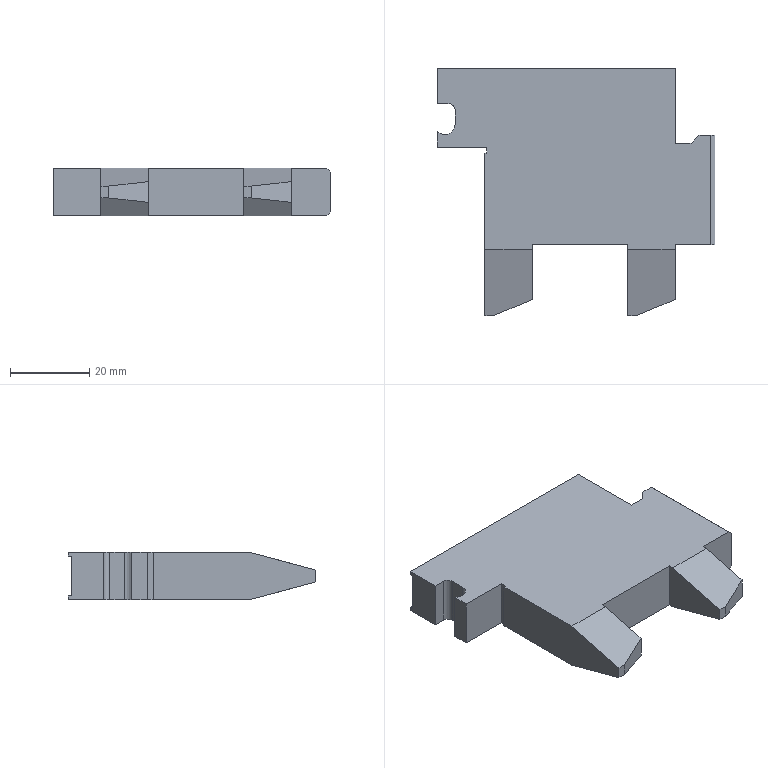Part | SolidWorks | features ICE 2, Chamfer 1, Extrusion 1 | 1 solid | 38 faces | box 70 x 62.5 x 12 mm | volume 33880 mm3 | plane 36 | cylinder 2 | commonest cylinder face diameters 3 x1 5 x1
STEP:
#1=CARTESIAN_POINT('',(0.,20.,-5.));
#2=VERTEX_POINT('',#1);
#3=CARTESIAN_POINT('',(0.,20.,-6.));
#4=VERTEX_POINT('',#3);
#5=CARTESIAN_POINT('',(0.,20.,6.));
#6=DIRECTION('',(0.,0.,-1.));
#7=VECTOR('',#6,1000.);
#8=LINE('',#5,#7);
#9=EDGE_CURVE('',#2,#4,#8,.T.);
#10=ORIENTED_EDGE('',*,*,#9,.F.);
#11=CARTESIAN_POINT('',(60.,20.,-5.));
#12=VERTEX_POINT('',#11);
#13=CARTESIAN_POINT('',(0.,20.,-5.));
#14=DIRECTION('',(-1.,0.,0.));
#15=VECTOR('',#14,1000.);
#16=LINE('',#13,#15);
#17=EDGE_CURVE('',#12,#2,#16,.T.);
#18=ORIENTED_EDGE('',*,*,#17,.F.);
#19=CARTESIAN_POINT('',(60.,20.,-6.));
#20=VERTEX_POINT('',#19);
#21=CARTESIAN_POINT('',(60.,20.,6.));
#22=DIRECTION('',(0.,0.,-1.));
#23=VECTOR('',#22,1000.);
#24=LINE('',#21,#23);
#25=EDGE_CURVE('',#12,#20,#24,.T.);
#26=ORIENTED_EDGE('',*,*,#25,.T.);
#27=CARTESIAN_POINT('',(0.,20.,-6.));
#28=DIRECTION('',(-1.,0.,0.));
#29=VECTOR('',#28,1000.);
#30=LINE('',#27,#29);
#31=EDGE_CURVE('',#20,#4,#30,.T.);
#32=ORIENTED_EDGE('',*,*,#31,.T.);
#33=EDGE_LOOP('',(#10,#18,#26,#32));
#34=FACE_OUTER_BOUND('',#33,.T.);
#35=CARTESIAN_POINT('',(0.,20.,6.));
#36=DIRECTION('',(0.,-1.,0.));
#37=DIRECTION('',(1.,0.,0.));
#38=AXIS2_PLACEMENT_3D('',#35,#36,#37);
#39=PLANE('',#38);
#40=ADVANCED_FACE('',(#34),#39,.F.);
#41=CARTESIAN_POINT('',(0.,0.,-6.));
#42=VERTEX_POINT('',#41);
#43=CARTESIAN_POINT('',(12.5,0.,-6.));
#44=VERTEX_POINT('',#43);
#45=CARTESIAN_POINT('',(12.5,0.,-6.));
#46=DIRECTION('',(1.,0.,0.));
#47=VECTOR('',#46,1000.);
#48=LINE('',#45,#47);
#49=EDGE_CURVE('',#42,#44,#48,.T.);
#50=ORIENTED_EDGE('',*,*,#49,.T.);
#51=CARTESIAN_POINT('',(12.5,0.,6.));
#52=VERTEX_POINT('',#51);
#53=CARTESIAN_POINT('',(12.5,0.,6.));
#54=DIRECTION('',(0.,0.,-1.));
#55=VECTOR('',#54,1000.);
#56=LINE('',#53,#55);
#57=EDGE_CURVE('',#52,#44,#56,.T.);
#58=ORIENTED_EDGE('',*,*,#57,.F.);
#59=CARTESIAN_POINT('',(0.,0.,6.));
#60=VERTEX_POINT('',#59);
#61=CARTESIAN_POINT('',(12.5,0.,6.));
#62=DIRECTION('',(1.,0.,0.));
#63=VECTOR('',#62,1000.);
#64=LINE('',#61,#63);
#65=EDGE_CURVE('',#60,#52,#64,.T.);
#66=ORIENTED_EDGE('',*,*,#65,.F.);
#67=CARTESIAN_POINT('',(0.,0.,6.));
#68=DIRECTION('',(0.,0.,-1.));
#69=VECTOR('',#68,1000.);
#70=LINE('',#67,#69);
#71=EDGE_CURVE('',#60,#42,#70,.T.);
#72=ORIENTED_EDGE('',*,*,#71,.T.);
#73=EDGE_LOOP('',(#50,#58,#66,#72));
#74=FACE_OUTER_BOUND('',#73,.T.);
#75=CARTESIAN_POINT('',(12.5,0.,6.));
#76=DIRECTION('',(0.,1.,0.));
#77=DIRECTION('',(-1.,0.,0.));
#78=AXIS2_PLACEMENT_3D('',#75,#76,#77);
#79=PLANE('',#78);
#80=ADVANCED_FACE('',(#74),#79,.F.);
#81=CARTESIAN_POINT('',(12.5,-1.5,-6.));
#82=VERTEX_POINT('',#81);
#83=CARTESIAN_POINT('',(12.5,0.,-6.));
#84=DIRECTION('',(0.,-1.,0.));
#85=VECTOR('',#84,1000.);
#86=LINE('',#83,#85);
#87=EDGE_CURVE('',#44,#82,#86,.T.);
#88=ORIENTED_EDGE('',*,*,#87,.T.);
#89=CARTESIAN_POINT('',(12.5,-1.5,6.));
#90=VERTEX_POINT('',#89);
#91=CARTESIAN_POINT('',(12.5,-1.5,6.));
#92=DIRECTION('',(0.,0.,-1.));
#93=VECTOR('',#92,1000.);
#94=LINE('',#91,#93);
#95=EDGE_CURVE('',#90,#82,#94,.T.);
#96=ORIENTED_EDGE('',*,*,#95,.F.);
#97=CARTESIAN_POINT('',(12.5,0.,6.));
#98=DIRECTION('',(0.,-1.,0.));
#99=VECTOR('',#98,1000.);
#100=LINE('',#97,#99);
#101=EDGE_CURVE('',#52,#90,#100,.T.);
#102=ORIENTED_EDGE('',*,*,#101,.F.);
#103=ORIENTED_EDGE('',*,*,#57,.T.);
#104=EDGE_LOOP('',(#88,#96,#102,#103));
#105=FACE_OUTER_BOUND('',#104,.T.);
#106=CARTESIAN_POINT('',(12.5,0.,6.));
#107=DIRECTION('',(1.,0.,0.));
#108=DIRECTION('',(0.,0.,-1.));
#109=AXIS2_PLACEMENT_3D('',#106,#107,#108);
#110=PLANE('',#109);
#111=ADVANCED_FACE('',(#105),#110,.F.);
#112=CARTESIAN_POINT('',(12.,-1.5,-6.));
#113=VERTEX_POINT('',#112);
#114=CARTESIAN_POINT('',(12.5,-1.5,-6.));
#115=DIRECTION('',(-1.,0.,0.));
#116=VECTOR('',#115,1000.);
#117=LINE('',#114,#116);
#118=EDGE_CURVE('',#82,#113,#117,.T.);
#119=ORIENTED_EDGE('',*,*,#118,.T.);
#120=CARTESIAN_POINT('',(12.,-1.5,6.));
#121=VERTEX_POINT('',#120);
#122=CARTESIAN_POINT('',(12.,-1.5,6.));
#123=DIRECTION('',(0.,0.,-1.));
#124=VECTOR('',#123,1000.);
#125=LINE('',#122,#124);
#126=EDGE_CURVE('',#121,#113,#125,.T.);
#127=ORIENTED_EDGE('',*,*,#126,.F.);
#128=CARTESIAN_POINT('',(12.5,-1.5,6.));
#129=DIRECTION('',(-1.,0.,0.));
#130=VECTOR('',#129,1000.);
#131=LINE('',#128,#130);
#132=EDGE_CURVE('',#90,#121,#131,.T.);
#133=ORIENTED_EDGE('',*,*,#132,.F.);
#134=ORIENTED_EDGE('',*,*,#95,.T.);
#135=EDGE_LOOP('',(#119,#127,#133,#134));
#136=FACE_OUTER_BOUND('',#135,.T.);
#137=CARTESIAN_POINT('',(12.5,-1.5,6.));
#138=DIRECTION('',(0.,-1.,0.));
#139=DIRECTION('',(0.,0.,-1.));
#140=AXIS2_PLACEMENT_3D('',#137,#138,#139);
#141=PLANE('',#140);
#142=ADVANCED_FACE('',(#136),#141,.F.);
#143=CARTESIAN_POINT('',(12.,-25.706,-6.));
#144=VERTEX_POINT('',#143);
#145=CARTESIAN_POINT('',(12.,-1.5,-6.));
#146=DIRECTION('',(0.,-1.,0.));
#147=VECTOR('',#146,1000.);
#148=LINE('',#145,#147);
#149=EDGE_CURVE('',#113,#144,#148,.T.);
#150=ORIENTED_EDGE('',*,*,#149,.T.);
#151=CARTESIAN_POINT('',(12.,-42.5,-1.5));
#152=VERTEX_POINT('',#151);
#153=CARTESIAN_POINT('',(12.,-42.5,-1.5));
#154=DIRECTION('',(0.,0.9659,-0.2588));
#155=VECTOR('',#154,1000.);
#156=LINE('',#153,#155);
#157=EDGE_CURVE('',#152,#144,#156,.T.);
#158=ORIENTED_EDGE('',*,*,#157,.F.);
#159=CARTESIAN_POINT('',(12.,-42.5,1.5));
#160=VERTEX_POINT('',#159);
#161=CARTESIAN_POINT('',(12.,-42.5,6.));
#162=DIRECTION('',(0.,0.,-1.));
#163=VECTOR('',#162,1000.);
#164=LINE('',#161,#163);
#165=EDGE_CURVE('',#160,#152,#164,.T.);
#166=ORIENTED_EDGE('',*,*,#165,.F.);
#167=CARTESIAN_POINT('',(12.,-25.706,6.));
#168=VERTEX_POINT('',#167);
#169=CARTESIAN_POINT('',(12.,-42.5,1.5));
#170=DIRECTION('',(0.,-0.9659,-0.2588));
#171=VECTOR('',#170,1000.);
#172=LINE('',#169,#171);
#173=EDGE_CURVE('',#168,#160,#172,.T.);
#174=ORIENTED_EDGE('',*,*,#173,.F.);
#175=CARTESIAN_POINT('',(12.,-1.5,6.));
#176=DIRECTION('',(0.,-1.,0.));
#177=VECTOR('',#176,1000.);
#178=LINE('',#175,#177);
#179=EDGE_CURVE('',#121,#168,#178,.T.);
#180=ORIENTED_EDGE('',*,*,#179,.F.);
#181=ORIENTED_EDGE('',*,*,#126,.T.);
#182=EDGE_LOOP('',(#150,#158,#166,#174,#180,#181));
#183=FACE_OUTER_BOUND('',#182,.T.);
#184=CARTESIAN_POINT('',(12.,-1.5,6.));
#185=DIRECTION('',(1.,0.,0.));
#186=DIRECTION('',(0.,1.,0.));
#187=AXIS2_PLACEMENT_3D('',#184,#185,#186);
#188=PLANE('',#187);
#189=ADVANCED_FACE('',(#183),#188,.F.);
#190=ORIENTED_EDGE('',*,*,#165,.T.);
#191=CARTESIAN_POINT('',(14.,-42.5,-1.5));
#192=VERTEX_POINT('',#191);
#193=CARTESIAN_POINT('',(70.,-42.5,-1.5));
#194=DIRECTION('',(-1.,0.,0.));
#195=VECTOR('',#194,1000.);
#196=LINE('',#193,#195);
#197=EDGE_CURVE('',#192,#152,#196,.T.);
#198=ORIENTED_EDGE('',*,*,#197,.F.);
#199=CARTESIAN_POINT('',(14.,-42.5,1.5));
#200=VERTEX_POINT('',#199);
#201=CARTESIAN_POINT('',(14.,-42.5,6.));
#202=DIRECTION('',(0.,0.,-1.));
#203=VECTOR('',#202,1000.);
#204=LINE('',#201,#203);
#205=EDGE_CURVE('',#200,#192,#204,.T.);
#206=ORIENTED_EDGE('',*,*,#205,.F.);
#207=CARTESIAN_POINT('',(70.,-42.5,1.5));
#208=DIRECTION('',(-1.,0.,0.));
#209=VECTOR('',#208,1000.);
#210=LINE('',#207,#209);
#211=EDGE_CURVE('',#200,#160,#210,.T.);
#212=ORIENTED_EDGE('',*,*,#211,.T.);
#213=EDGE_LOOP('',(#190,#198,#206,#212));
#214=FACE_OUTER_BOUND('',#213,.T.);
#215=CARTESIAN_POINT('',(14.,-42.5,6.));
#216=DIRECTION('',(0.,1.,0.));
#217=DIRECTION('',(0.,0.,1.));
#218=AXIS2_PLACEMENT_3D('',#215,#216,#217);
#219=PLANE('',#218);
#220=ADVANCED_FACE('',(#214),#219,.F.);
#221=ORIENTED_EDGE('',*,*,#205,.T.);
#222=CARTESIAN_POINT('',(24.,-38.358,-2.61));
#223=VERTEX_POINT('',#222);
#224=CARTESIAN_POINT('',(23.193,-38.692,-2.52));
#225=DIRECTION('',(0.9191,0.3807,-0.102));
#226=VECTOR('',#225,1000.);
#227=LINE('',#224,#226);
#228=EDGE_CURVE('',#192,#223,#227,.T.);
#229=ORIENTED_EDGE('',*,*,#228,.T.);
#230=CARTESIAN_POINT('',(24.,-38.358,2.61));
#231=VERTEX_POINT('',#230);
#232=CARTESIAN_POINT('',(24.,-38.358,6.));
#233=DIRECTION('',(0.,0.,-1.));
#234=VECTOR('',#233,1000.);
#235=LINE('',#232,#234);
#236=EDGE_CURVE('',#231,#223,#235,.T.);
#237=ORIENTED_EDGE('',*,*,#236,.F.);
#238=CARTESIAN_POINT('',(24.318,-38.226,2.645));
#239=DIRECTION('',(-0.9191,-0.3807,-0.102));
#240=VECTOR('',#239,1000.);
#241=LINE('',#238,#240);
#242=EDGE_CURVE('',#231,#200,#241,.T.);
#243=ORIENTED_EDGE('',*,*,#242,.T.);
#244=EDGE_LOOP('',(#221,#229,#237,#243));
#245=FACE_OUTER_BOUND('',#244,.T.);
#246=CARTESIAN_POINT('',(24.,-38.358,6.));
#247=DIRECTION('',(-0.3827,0.9239,0.));
#248=DIRECTION('',(-0.9239,-0.3827,0.));
#249=AXIS2_PLACEMENT_3D('',#246,#247,#248);
#250=PLANE('',#249);
#251=ADVANCED_FACE('',(#245),#250,.F.);
#252=ORIENTED_EDGE('',*,*,#236,.T.);
#253=CARTESIAN_POINT('',(24.,-25.706,-6.));
#254=VERTEX_POINT('',#253);
#255=CARTESIAN_POINT('',(24.,-27.581,-5.498));
#256=DIRECTION('',(0.,0.9659,-0.2588));
#257=VECTOR('',#256,1000.);
#258=LINE('',#255,#257);
#259=EDGE_CURVE('',#223,#254,#258,.T.);
#260=ORIENTED_EDGE('',*,*,#259,.T.);
#261=CARTESIAN_POINT('',(24.,-24.5,-6.));
#262=VERTEX_POINT('',#261);
#263=CARTESIAN_POINT('',(24.,-24.5,-6.));
#264=DIRECTION('',(0.,1.,0.));
#265=VECTOR('',#264,1000.);
#266=LINE('',#263,#265);
#267=EDGE_CURVE('',#254,#262,#266,.T.);
#268=ORIENTED_EDGE('',*,*,#267,.T.);
#269=CARTESIAN_POINT('',(24.,-24.5,6.));
#270=VERTEX_POINT('',#269);
#271=CARTESIAN_POINT('',(24.,-24.5,6.));
#272=DIRECTION('',(0.,0.,-1.));
#273=VECTOR('',#272,1000.);
#274=LINE('',#271,#273);
#275=EDGE_CURVE('',#270,#262,#274,.T.);
#276=ORIENTED_EDGE('',*,*,#275,.F.);
#277=CARTESIAN_POINT('',(24.,-25.706,6.));
#278=VERTEX_POINT('',#277);
#279=CARTESIAN_POINT('',(24.,-24.5,6.));
#280=DIRECTION('',(0.,1.,0.));
#281=VECTOR('',#280,1000.);
#282=LINE('',#279,#281);
#283=EDGE_CURVE('',#278,#270,#282,.T.);
#284=ORIENTED_EDGE('',*,*,#283,.F.);
#285=CARTESIAN_POINT('',(24.,-24.581,6.301));
#286=DIRECTION('',(0.,-0.9659,-0.2588));
#287=VECTOR('',#286,1000.);
#288=LINE('',#285,#287);
#289=EDGE_CURVE('',#278,#231,#288,.T.);
#290=ORIENTED_EDGE('',*,*,#289,.T.);
#291=EDGE_LOOP('',(#252,#260,#268,#276,#284,#290));
#292=FACE_OUTER_BOUND('',#291,.T.);
#293=CARTESIAN_POINT('',(24.,-24.5,6.));
#294=DIRECTION('',(-1.,0.,0.));
#295=DIRECTION('',(0.,0.,1.));
#296=AXIS2_PLACEMENT_3D('',#293,#294,#295);
#297=PLANE('',#296);
#298=ADVANCED_FACE('',(#292),#297,.F.);
#299=CARTESIAN_POINT('',(48.,-24.5,-6.));
#300=VERTEX_POINT('',#299);
#301=CARTESIAN_POINT('',(48.,-24.5,-6.));
#302=DIRECTION('',(1.,0.,0.));
#303=VECTOR('',#302,1000.);
#304=LINE('',#301,#303);
#305=EDGE_CURVE('',#262,#300,#304,.T.);
#306=ORIENTED_EDGE('',*,*,#305,.T.);
#307=CARTESIAN_POINT('',(48.,-24.5,6.));
#308=VERTEX_POINT('',#307);
#309=CARTESIAN_POINT('',(48.,-24.5,6.));
#310=DIRECTION('',(0.,0.,-1.));
#311=VECTOR('',#310,1000.);
#312=LINE('',#309,#311);
#313=EDGE_CURVE('',#308,#300,#312,.T.);
#314=ORIENTED_EDGE('',*,*,#313,.F.);
#315=CARTESIAN_POINT('',(48.,-24.5,6.));
#316=DIRECTION('',(1.,0.,0.));
#317=VECTOR('',#316,1000.);
#318=LINE('',#315,#317);
#319=EDGE_CURVE('',#270,#308,#318,.T.);
#320=ORIENTED_EDGE('',*,*,#319,.F.);
#321=ORIENTED_EDGE('',*,*,#275,.T.);
#322=EDGE_LOOP('',(#306,#314,#320,#321));
#323=FACE_OUTER_BOUND('',#322,.T.);
#324=CARTESIAN_POINT('',(48.,-24.5,6.));
#325=DIRECTION('',(0.,1.,0.));
#326=DIRECTION('',(-1.,0.,0.));
#327=AXIS2_PLACEMENT_3D('',#324,#325,#326);
#328=PLANE('',#327);
#329=ADVANCED_FACE('',(#323),#328,.F.);
#330=CARTESIAN_POINT('',(48.,-25.706,-6.));
#331=VERTEX_POINT('',#330);
#332=CARTESIAN_POINT('',(48.,-42.5,-6.));
#333=DIRECTION('',(0.,-1.,0.));
#334=VECTOR('',#333,1000.);
#335=LINE('',#332,#334);
#336=EDGE_CURVE('',#300,#331,#335,.T.);
#337=ORIENTED_EDGE('',*,*,#336,.T.);
#338=CARTESIAN_POINT('',(48.,-42.5,-1.5));
#339=VERTEX_POINT('',#338);
#340=CARTESIAN_POINT('',(48.,-44.375,-0.9976));
#341=DIRECTION('',(0.,-0.9659,0.2588));
#342=VECTOR('',#341,1000.);
#343=LINE('',#340,#342);
#344=EDGE_CURVE('',#331,#339,#343,.T.);
#345=ORIENTED_EDGE('',*,*,#344,.T.);
#346=CARTESIAN_POINT('',(48.,-42.5,1.5));
#347=VERTEX_POINT('',#346);
#348=CARTESIAN_POINT('',(48.,-42.5,6.));
#349=DIRECTION('',(0.,0.,-1.));
#350=VECTOR('',#349,1000.);
#351=LINE('',#348,#350);
#352=EDGE_CURVE('',#347,#339,#351,.T.);
#353=ORIENTED_EDGE('',*,*,#352,.F.);
#354=CARTESIAN_POINT('',(48.,-25.706,6.));
#355=VERTEX_POINT('',#354);
#356=CARTESIAN_POINT('',(48.,-41.375,1.801));
#357=DIRECTION('',(0.,0.9659,0.2588));
#358=VECTOR('',#357,1000.);
#359=LINE('',#356,#358);
#360=EDGE_CURVE('',#347,#355,#359,.T.);
#361=ORIENTED_EDGE('',*,*,#360,.T.);
#362=CARTESIAN_POINT('',(48.,-42.5,6.));
#363=DIRECTION('',(0.,-1.,0.));
#364=VECTOR('',#363,1000.);
#365=LINE('',#362,#364);
#366=EDGE_CURVE('',#308,#355,#365,.T.);
#367=ORIENTED_EDGE('',*,*,#366,.F.);
#368=ORIENTED_EDGE('',*,*,#313,.T.);
#369=EDGE_LOOP('',(#337,#345,#353,#361,#367,#368));
#370=FACE_OUTER_BOUND('',#369,.T.);
#371=CARTESIAN_POINT('',(48.,-42.5,6.));
#372=DIRECTION('',(1.,0.,0.));
#373=DIRECTION('',(0.,0.,-1.));
#374=AXIS2_PLACEMENT_3D('',#371,#372,#373);
#375=PLANE('',#374);
#376=ADVANCED_FACE('',(#370),#375,.F.);
#377=ORIENTED_EDGE('',*,*,#352,.T.);
#378=CARTESIAN_POINT('',(50.,-42.5,-1.5));
#379=VERTEX_POINT('',#378);
#380=CARTESIAN_POINT('',(70.,-42.5,-1.5));
#381=DIRECTION('',(-1.,0.,0.));
#382=VECTOR('',#381,1000.);
#383=LINE('',#380,#382);
#384=EDGE_CURVE('',#379,#339,#383,.T.);
#385=ORIENTED_EDGE('',*,*,#384,.F.);
#386=CARTESIAN_POINT('',(50.,-42.5,1.5));
#387=VERTEX_POINT('',#386);
#388=CARTESIAN_POINT('',(50.,-42.5,6.));
#389=DIRECTION('',(0.,0.,-1.));
#390=VECTOR('',#389,1000.);
#391=LINE('',#388,#390);
#392=EDGE_CURVE('',#387,#379,#391,.T.);
#393=ORIENTED_EDGE('',*,*,#392,.F.);
#394=CARTESIAN_POINT('',(70.,-42.5,1.5));
#395=DIRECTION('',(-1.,0.,0.));
#396=VECTOR('',#395,1000.);
#397=LINE('',#394,#396);
#398=EDGE_CURVE('',#387,#347,#397,.T.);
#399=ORIENTED_EDGE('',*,*,#398,.T.);
#400=EDGE_LOOP('',(#377,#385,#393,#399));
#401=FACE_OUTER_BOUND('',#400,.T.);
#402=CARTESIAN_POINT('',(50.,-42.5,6.));
#403=DIRECTION('',(0.,1.,0.));
#404=DIRECTION('',(-1.,0.,0.));
#405=AXIS2_PLACEMENT_3D('',#402,#403,#404);
#406=PLANE('',#405);
#407=ADVANCED_FACE('',(#401),#406,.F.);
#408=ORIENTED_EDGE('',*,*,#392,.T.);
#409=CARTESIAN_POINT('',(60.,-38.358,-2.61));
#410=VERTEX_POINT('',#409);
#411=CARTESIAN_POINT('',(59.193,-38.692,-2.52));
#412=DIRECTION('',(0.9191,0.3807,-0.102));
#413=VECTOR('',#412,1000.);
#414=LINE('',#411,#413);
#415=EDGE_CURVE('',#379,#410,#414,.T.);
#416=ORIENTED_EDGE('',*,*,#415,.T.);
#417=CARTESIAN_POINT('',(60.,-38.358,2.61));
#418=VERTEX_POINT('',#417);
#419=CARTESIAN_POINT('',(60.,-38.358,6.));
#420=DIRECTION('',(0.,0.,-1.));
#421=VECTOR('',#420,1000.);
#422=LINE('',#419,#421);
#423=EDGE_CURVE('',#418,#410,#422,.T.);
#424=ORIENTED_EDGE('',*,*,#423,.F.);
#425=CARTESIAN_POINT('',(60.318,-38.226,2.645));
#426=DIRECTION('',(-0.9191,-0.3807,-0.102));
#427=VECTOR('',#426,1000.);
#428=LINE('',#425,#427);
#429=EDGE_CURVE('',#418,#387,#428,.T.);
#430=ORIENTED_EDGE('',*,*,#429,.T.);
#431=EDGE_LOOP('',(#408,#416,#424,#430));
#432=FACE_OUTER_BOUND('',#431,.T.);
#433=CARTESIAN_POINT('',(60.,-38.358,6.));
#434=DIRECTION('',(-0.3827,0.9239,0.));
#435=DIRECTION('',(-0.9239,-0.3827,0.));
#436=AXIS2_PLACEMENT_3D('',#433,#434,#435);
#437=PLANE('',#436);
#438=ADVANCED_FACE('',(#432),#437,.F.);
#439=ORIENTED_EDGE('',*,*,#423,.T.);
#440=CARTESIAN_POINT('',(60.,-25.706,-6.));
#441=VERTEX_POINT('',#440);
#442=CARTESIAN_POINT('',(60.,-40.51,-2.033));
#443=DIRECTION('',(0.,0.9659,-0.2588));
#444=VECTOR('',#443,1000.);
#445=LINE('',#442,#444);
#446=EDGE_CURVE('',#410,#441,#445,.T.);
#447=ORIENTED_EDGE('',*,*,#446,.T.);
#448=CARTESIAN_POINT('',(60.,-24.5,-6.));
#449=VERTEX_POINT('',#448);
#450=CARTESIAN_POINT('',(60.,-38.358,-6.));
#451=DIRECTION('',(0.,1.,0.));
#452=VECTOR('',#451,1000.);
#453=LINE('',#450,#452);
#454=EDGE_CURVE('',#441,#449,#453,.T.);
#455=ORIENTED_EDGE('',*,*,#454,.T.);
#456=CARTESIAN_POINT('',(60.,-24.5,6.));
#457=VERTEX_POINT('',#456);
#458=CARTESIAN_POINT('',(60.,-24.5,6.));
#459=DIRECTION('',(0.,0.,-1.));
#460=VECTOR('',#459,1000.);
#461=LINE('',#458,#460);
#462=EDGE_CURVE('',#457,#449,#461,.T.);
#463=ORIENTED_EDGE('',*,*,#462,.F.);
#464=CARTESIAN_POINT('',(60.,-25.706,6.));
#465=VERTEX_POINT('',#464);
#466=CARTESIAN_POINT('',(60.,-38.358,6.));
#467=DIRECTION('',(0.,1.,0.));
#468=VECTOR('',#467,1000.);
#469=LINE('',#466,#468);
#470=EDGE_CURVE('',#465,#457,#469,.T.);
#471=ORIENTED_EDGE('',*,*,#470,.F.);
#472=CARTESIAN_POINT('',(60.,-37.51,2.837));
#473=DIRECTION('',(0.,-0.9659,-0.2588));
#474=VECTOR('',#473,1000.);
#475=LINE('',#472,#474);
#476=EDGE_CURVE('',#465,#418,#475,.T.);
#477=ORIENTED_EDGE('',*,*,#476,.T.);
#478=EDGE_LOOP('',(#439,#447,#455,#463,#471,#477));
#479=FACE_OUTER_BOUND('',#478,.T.);
#480=CARTESIAN_POINT('',(60.,-38.358,6.));
#481=DIRECTION('',(-1.,0.,0.));
#482=DIRECTION('',(0.,0.,1.));
#483=AXIS2_PLACEMENT_3D('',#480,#481,#482);
#484=PLANE('',#483);
#485=ADVANCED_FACE('',(#479),#484,.F.);
#486=CARTESIAN_POINT('',(69.,-24.5,-6.));
#487=VERTEX_POINT('',#486);
#488=CARTESIAN_POINT('',(70.,-24.5,-6.));
#489=DIRECTION('',(1.,0.,0.));
#490=VECTOR('',#489,1000.);
#491=LINE('',#488,#490);
#492=EDGE_CURVE('',#449,#487,#491,.T.);
#493=ORIENTED_EDGE('',*,*,#492,.T.);
#494=CARTESIAN_POINT('',(70.,-24.5,-5.));
#495=VERTEX_POINT('',#494);
#496=CARTESIAN_POINT('',(70.,-24.5,-5.));
#497=DIRECTION('',(0.7071,0.,0.7071));
#498=VECTOR('',#497,1000.);
#499=LINE('',#496,#498);
#500=EDGE_CURVE('',#487,#495,#499,.T.);
#501=ORIENTED_EDGE('',*,*,#500,.T.);
#502=CARTESIAN_POINT('',(70.,-24.5,5.));
#503=VERTEX_POINT('',#502);
#504=CARTESIAN_POINT('',(70.,-24.5,6.));
#505=DIRECTION('',(0.,0.,-1.));
#506=VECTOR('',#505,1000.);
#507=LINE('',#504,#506);
#508=EDGE_CURVE('',#503,#495,#507,.T.);
#509=ORIENTED_EDGE('',*,*,#508,.F.);
#510=CARTESIAN_POINT('',(69.,-24.5,6.));
#511=VERTEX_POINT('',#510);
#512=CARTESIAN_POINT('',(69.,-24.5,6.));
#513=DIRECTION('',(-0.7071,0.,0.7071));
#514=VECTOR('',#513,1000.);
#515=LINE('',#512,#514);
#516=EDGE_CURVE('',#503,#511,#515,.T.);
#517=ORIENTED_EDGE('',*,*,#516,.T.);
#518=CARTESIAN_POINT('',(70.,-24.5,6.));
#519=DIRECTION('',(1.,0.,0.));
#520=VECTOR('',#519,1000.);
#521=LINE('',#518,#520);
#522=EDGE_CURVE('',#457,#511,#521,.T.);
#523=ORIENTED_EDGE('',*,*,#522,.F.);
#524=ORIENTED_EDGE('',*,*,#462,.T.);
#525=EDGE_LOOP('',(#493,#501,#509,#517,#523,#524));
#526=FACE_OUTER_BOUND('',#525,.T.);
#527=CARTESIAN_POINT('',(70.,-24.5,6.));
#528=DIRECTION('',(0.,1.,0.));
#529=DIRECTION('',(-1.,0.,0.));
#530=AXIS2_PLACEMENT_3D('',#527,#528,#529);
#531=PLANE('',#530);
#532=ADVANCED_FACE('',(#526),#531,.F.);
#533=ORIENTED_EDGE('',*,*,#508,.T.);
#534=CARTESIAN_POINT('',(70.,3.,-5.));
#535=VERTEX_POINT('',#534);
#536=CARTESIAN_POINT('',(70.,3.,-5.));
#537=DIRECTION('',(0.,1.,0.));
#538=VECTOR('',#537,1000.);
#539=LINE('',#536,#538);
#540=EDGE_CURVE('',#495,#535,#539,.T.);
#541=ORIENTED_EDGE('',*,*,#540,.T.);
#542=CARTESIAN_POINT('',(70.,3.,5.));
#543=VERTEX_POINT('',#542);
#544=CARTESIAN_POINT('',(70.,3.,6.));
#545=DIRECTION('',(0.,0.,-1.));
#546=VECTOR('',#545,1000.);
#547=LINE('',#544,#546);
#548=EDGE_CURVE('',#543,#535,#547,.T.);
#549=ORIENTED_EDGE('',*,*,#548,.F.);
#550=CARTESIAN_POINT('',(70.,-24.5,5.));
#551=DIRECTION('',(0.,-1.,0.));
#552=VECTOR('',#551,1000.);
#553=LINE('',#550,#552);
#554=EDGE_CURVE('',#543,#503,#553,.T.);
#555=ORIENTED_EDGE('',*,*,#554,.T.);
#556=EDGE_LOOP('',(#533,#541,#549,#555));
#557=FACE_OUTER_BOUND('',#556,.T.);
#558=CARTESIAN_POINT('',(70.,3.,6.));
#559=DIRECTION('',(-1.,0.,0.));
#560=DIRECTION('',(0.,-1.,0.));
#561=AXIS2_PLACEMENT_3D('',#558,#559,#560);
#562=PLANE('',#561);
#563=ADVANCED_FACE('',(#557),#562,.F.);
#564=ORIENTED_EDGE('',*,*,#548,.T.);
#565=CARTESIAN_POINT('',(69.,3.,-6.));
#566=VERTEX_POINT('',#565);
#567=CARTESIAN_POINT('',(70.,3.,-5.));
#568=DIRECTION('',(-0.7071,0.,-0.7071));
#569=VECTOR('',#568,1000.);
#570=LINE('',#567,#569);
#571=EDGE_CURVE('',#535,#566,#570,.T.);
#572=ORIENTED_EDGE('',*,*,#571,.T.);
#573=CARTESIAN_POINT('',(66.,3.,-6.));
#574=VERTEX_POINT('',#573);
#575=CARTESIAN_POINT('',(66.,3.,-6.));
#576=DIRECTION('',(-1.,0.,0.));
#577=VECTOR('',#576,1000.);
#578=LINE('',#575,#577);
#579=EDGE_CURVE('',#566,#574,#578,.T.);
#580=ORIENTED_EDGE('',*,*,#579,.T.);
#581=CARTESIAN_POINT('',(66.,3.,6.));
#582=VERTEX_POINT('',#581);
#583=CARTESIAN_POINT('',(66.,3.,6.));
#584=DIRECTION('',(0.,0.,-1.));
#585=VECTOR('',#584,1000.);
#586=LINE('',#583,#585);
#587=EDGE_CURVE('',#582,#574,#586,.T.);
#588=ORIENTED_EDGE('',*,*,#587,.F.);
#589=CARTESIAN_POINT('',(69.,3.,6.));
#590=VERTEX_POINT('',#589);
#591=CARTESIAN_POINT('',(66.,3.,6.));
#592=DIRECTION('',(-1.,0.,0.));
#593=VECTOR('',#592,1000.);
#594=LINE('',#591,#593);
#595=EDGE_CURVE('',#590,#582,#594,.T.);
#596=ORIENTED_EDGE('',*,*,#595,.F.);
#597=CARTESIAN_POINT('',(69.,3.,6.));
#598=DIRECTION('',(0.7071,0.,-0.7071));
#599=VECTOR('',#598,1000.);
#600=LINE('',#597,#599);
#601=EDGE_CURVE('',#590,#543,#600,.T.);
#602=ORIENTED_EDGE('',*,*,#601,.T.);
#603=EDGE_LOOP('',(#564,#572,#580,#588,#596,#602));
#604=FACE_OUTER_BOUND('',#603,.T.);
#605=CARTESIAN_POINT('',(66.,3.,6.));
#606=DIRECTION('',(0.,-1.,0.));
#607=DIRECTION('',(1.,0.,0.));
#608=AXIS2_PLACEMENT_3D('',#605,#606,#607);
#609=PLANE('',#608);
#610=ADVANCED_FACE('',(#604),#609,.F.);
#611=CARTESIAN_POINT('',(64.,1.,-6.));
#612=VERTEX_POINT('',#611);
#613=CARTESIAN_POINT('',(64.,1.,-6.));
#614=DIRECTION('',(-0.7071,-0.7071,0.));
#615=VECTOR('',#614,1000.);
#616=LINE('',#613,#615);
#617=EDGE_CURVE('',#574,#612,#616,.T.);
#618=ORIENTED_EDGE('',*,*,#617,.T.);
#619=CARTESIAN_POINT('',(64.,1.,6.));
#620=VERTEX_POINT('',#619);
#621=CARTESIAN_POINT('',(64.,1.,6.));
#622=DIRECTION('',(0.,0.,-1.));
#623=VECTOR('',#622,1000.);
#624=LINE('',#621,#623);
#625=EDGE_CURVE('',#620,#612,#624,.T.);
#626=ORIENTED_EDGE('',*,*,#625,.F.);
#627=CARTESIAN_POINT('',(64.,1.,6.));
#628=DIRECTION('',(-0.7071,-0.7071,0.));
#629=VECTOR('',#628,1000.);
#630=LINE('',#627,#629);
#631=EDGE_CURVE('',#582,#620,#630,.T.);
#632=ORIENTED_EDGE('',*,*,#631,.F.);
#633=ORIENTED_EDGE('',*,*,#587,.T.);
#634=EDGE_LOOP('',(#618,#626,#632,#633));
#635=FACE_OUTER_BOUND('',#634,.T.);
#636=CARTESIAN_POINT('',(64.,1.,6.));
#637=DIRECTION('',(0.7071,-0.7071,0.));
#638=DIRECTION('',(0.7071,0.7071,0.));
#639=AXIS2_PLACEMENT_3D('',#636,#637,#638);
#640=PLANE('',#639);
#641=ADVANCED_FACE('',(#635),#640,.F.);
#642=CARTESIAN_POINT('',(60.,1.,-6.));
#643=VERTEX_POINT('',#642);
#644=CARTESIAN_POINT('',(60.,1.,-6.));
#645=DIRECTION('',(-1.,0.,0.));
#646=VECTOR('',#645,1000.);
#647=LINE('',#644,#646);
#648=EDGE_CURVE('',#612,#643,#647,.T.);
#649=ORIENTED_EDGE('',*,*,#648,.T.);
#650=CARTESIAN_POINT('',(60.,1.,6.));
#651=VERTEX_POINT('',#650);
#652=CARTESIAN_POINT('',(60.,1.,6.));
#653=DIRECTION('',(0.,0.,-1.));
#654=VECTOR('',#653,1000.);
#655=LINE('',#652,#654);
#656=EDGE_CURVE('',#651,#643,#655,.T.);
#657=ORIENTED_EDGE('',*,*,#656,.F.);
#658=CARTESIAN_POINT('',(60.,1.,6.));
#659=DIRECTION('',(-1.,0.,0.));
#660=VECTOR('',#659,1000.);
#661=LINE('',#658,#660);
#662=EDGE_CURVE('',#620,#651,#661,.T.);
#663=ORIENTED_EDGE('',*,*,#662,.F.);
#664=ORIENTED_EDGE('',*,*,#625,.T.);
#665=EDGE_LOOP('',(#649,#657,#663,#664));
#666=FACE_OUTER_BOUND('',#665,.T.);
#667=CARTESIAN_POINT('',(60.,1.,6.));
#668=DIRECTION('',(0.,-1.,0.));
#669=DIRECTION('',(1.,0.,0.));
#670=AXIS2_PLACEMENT_3D('',#667,#668,#669);
#671=PLANE('',#670);
#672=ADVANCED_FACE('',(#666),#671,.F.);
#673=ORIENTED_EDGE('',*,*,#25,.F.);
#674=CARTESIAN_POINT('',(60.,19.,-5.));
#675=VERTEX_POINT('',#674);
#676=CARTESIAN_POINT('',(60.,19.,-5.));
#677=DIRECTION('',(0.,1.,0.));
#678=VECTOR('',#677,1000.);
#679=LINE('',#676,#678);
#680=EDGE_CURVE('',#675,#12,#679,.T.);
#681=ORIENTED_EDGE('',*,*,#680,.F.);
#682=CARTESIAN_POINT('',(60.,19.,5.));
#683=VERTEX_POINT('',#682);
#684=CARTESIAN_POINT('',(60.,19.,-5.));
#685=DIRECTION('',(0.,0.,-1.));
#686=VECTOR('',#685,1000.);
#687=LINE('',#684,#686);
#688=EDGE_CURVE('',#683,#675,#687,.T.);
#689=ORIENTED_EDGE('',*,*,#688,.F.);
#690=CARTESIAN_POINT('',(60.,20.,5.));
#691=VERTEX_POINT('',#690);
#692=CARTESIAN_POINT('',(60.,19.,5.));
#693=DIRECTION('',(0.,1.,0.));
#694=VECTOR('',#693,1000.);
#695=LINE('',#692,#694);
#696=EDGE_CURVE('',#683,#691,#695,.T.);
#697=ORIENTED_EDGE('',*,*,#696,.T.);
#698=CARTESIAN_POINT('',(60.,20.,6.));
#699=VERTEX_POINT('',#698);
#700=CARTESIAN_POINT('',(60.,20.,6.));
#701=DIRECTION('',(0.,0.,-1.));
#702=VECTOR('',#701,1000.);
#703=LINE('',#700,#702);
#704=EDGE_CURVE('',#699,#691,#703,.T.);
#705=ORIENTED_EDGE('',*,*,#704,.F.);
#706=CARTESIAN_POINT('',(60.,20.,6.));
#707=DIRECTION('',(0.,1.,0.));
#708=VECTOR('',#707,1000.);
#709=LINE('',#706,#708);
#710=EDGE_CURVE('',#651,#699,#709,.T.);
#711=ORIENTED_EDGE('',*,*,#710,.F.);
#712=ORIENTED_EDGE('',*,*,#656,.T.);
#713=CARTESIAN_POINT('',(60.,20.,-6.));
#714=DIRECTION('',(0.,1.,0.));
#715=VECTOR('',#714,1000.);
#716=LINE('',#713,#715);
#717=EDGE_CURVE('',#643,#20,#716,.T.);
#718=ORIENTED_EDGE('',*,*,#717,.T.);
#719=EDGE_LOOP('',(#673,#681,#689,#697,#705,#711,#712,#718));
#720=FACE_OUTER_BOUND('',#719,.T.);
#721=CARTESIAN_POINT('',(60.,20.,6.));
#722=DIRECTION('',(-1.,0.,0.));
#723=DIRECTION('',(0.,0.,1.));
#724=AXIS2_PLACEMENT_3D('',#721,#722,#723);
#725=PLANE('',#724);
#726=ADVANCED_FACE('',(#720),#725,.F.);
#727=ORIENTED_EDGE('',*,*,#704,.T.);
#728=CARTESIAN_POINT('',(0.,20.,5.));
#729=VERTEX_POINT('',#728);
#730=CARTESIAN_POINT('',(0.,20.,5.));
#731=DIRECTION('',(1.,0.,0.));
#732=VECTOR('',#731,1000.);
#733=LINE('',#730,#732);
#734=EDGE_CURVE('',#729,#691,#733,.T.);
#735=ORIENTED_EDGE('',*,*,#734,.F.);
#736=CARTESIAN_POINT('',(0.,20.,6.));
#737=VERTEX_POINT('',#736);
#738=CARTESIAN_POINT('',(0.,20.,6.));
#739=DIRECTION('',(0.,0.,-1.));
#740=VECTOR('',#739,1000.);
#741=LINE('',#738,#740);
#742=EDGE_CURVE('',#737,#729,#741,.T.);
#743=ORIENTED_EDGE('',*,*,#742,.F.);
#744=CARTESIAN_POINT('',(0.,20.,6.));
#745=DIRECTION('',(-1.,0.,0.));
#746=VECTOR('',#745,1000.);
#747=LINE('',#744,#746);
#748=EDGE_CURVE('',#699,#737,#747,.T.);
#749=ORIENTED_EDGE('',*,*,#748,.F.);
#750=EDGE_LOOP('',(#727,#735,#743,#749));
#751=FACE_OUTER_BOUND('',#750,.T.);
#752=CARTESIAN_POINT('',(0.,20.,6.));
#753=DIRECTION('',(0.,-1.,0.));
#754=DIRECTION('',(1.,0.,0.));
#755=AXIS2_PLACEMENT_3D('',#752,#753,#754);
#756=PLANE('',#755);
#757=ADVANCED_FACE('',(#751),#756,.F.);
#758=CARTESIAN_POINT('',(0.,19.,-5.));
#759=VERTEX_POINT('',#758);
#760=CARTESIAN_POINT('',(0.,19.,5.));
#761=VERTEX_POINT('',#760);
#762=CARTESIAN_POINT('',(0.,19.,-5.));
#763=DIRECTION('',(0.,0.,1.));
#764=VECTOR('',#763,1000.);
#765=LINE('',#762,#764);
#766=EDGE_CURVE('',#759,#761,#765,.T.);
#767=ORIENTED_EDGE('',*,*,#766,.F.);
#768=CARTESIAN_POINT('',(0.,19.,-5.));
#769=DIRECTION('',(0.,1.,0.));
#770=VECTOR('',#769,1000.);
#771=LINE('',#768,#770);
#772=EDGE_CURVE('',#759,#2,#771,.T.);
#773=ORIENTED_EDGE('',*,*,#772,.T.);
#774=ORIENTED_EDGE('',*,*,#9,.T.);
#775=CARTESIAN_POINT('',(0.,11.,-6.));
#776=VERTEX_POINT('',#775);
#777=CARTESIAN_POINT('',(0.,11.,-6.));
#778=DIRECTION('',(0.,-1.,0.));
#779=VECTOR('',#778,1000.);
#780=LINE('',#777,#779);
#781=EDGE_CURVE('',#4,#776,#780,.T.);
#782=ORIENTED_EDGE('',*,*,#781,.T.);
#783=CARTESIAN_POINT('',(0.,11.,6.));
#784=VERTEX_POINT('',#783);
#785=CARTESIAN_POINT('',(0.,11.,6.));
#786=DIRECTION('',(0.,0.,-1.));
#787=VECTOR('',#786,1000.);
#788=LINE('',#785,#787);
#789=EDGE_CURVE('',#784,#776,#788,.T.);
#790=ORIENTED_EDGE('',*,*,#789,.F.);
#791=CARTESIAN_POINT('',(0.,11.,6.));
#792=DIRECTION('',(0.,-1.,0.));
#793=VECTOR('',#792,1000.);
#794=LINE('',#791,#793);
#795=EDGE_CURVE('',#737,#784,#794,.T.);
#796=ORIENTED_EDGE('',*,*,#795,.F.);
#797=ORIENTED_EDGE('',*,*,#742,.T.);
#798=CARTESIAN_POINT('',(0.,19.,5.));
#799=DIRECTION('',(0.,1.,0.));
#800=VECTOR('',#799,1000.);
#801=LINE('',#798,#800);
#802=EDGE_CURVE('',#761,#729,#801,.T.);
#803=ORIENTED_EDGE('',*,*,#802,.F.);
#804=EDGE_LOOP('',(#767,#773,#774,#782,#790,#796,#797,#803));
#805=FACE_OUTER_BOUND('',#804,.T.);
#806=CARTESIAN_POINT('',(0.,11.,6.));
#807=DIRECTION('',(1.,0.,0.));
#808=DIRECTION('',(0.,0.,-1.));
#809=AXIS2_PLACEMENT_3D('',#806,#807,#808);
#810=PLANE('',#809);
#811=ADVANCED_FACE('',(#805),#810,.F.);
#812=CARTESIAN_POINT('',(3.,11.,-6.));
#813=VERTEX_POINT('',#812);
#814=CARTESIAN_POINT('',(3.,11.,-6.));
#815=DIRECTION('',(1.,0.,0.));
#816=VECTOR('',#815,1000.);
#817=LINE('',#814,#816);
#818=EDGE_CURVE('',#776,#813,#817,.T.);
#819=ORIENTED_EDGE('',*,*,#818,.T.);
#820=CARTESIAN_POINT('',(3.,11.,6.));
#821=VERTEX_POINT('',#820);
#822=CARTESIAN_POINT('',(3.,11.,6.));
#823=DIRECTION('',(0.,0.,-1.));
#824=VECTOR('',#823,1000.);
#825=LINE('',#822,#824);
#826=EDGE_CURVE('',#821,#813,#825,.T.);
#827=ORIENTED_EDGE('',*,*,#826,.F.);
#828=CARTESIAN_POINT('',(3.,11.,6.));
#829=DIRECTION('',(1.,0.,0.));
#830=VECTOR('',#829,1000.);
#831=LINE('',#828,#830);
#832=EDGE_CURVE('',#784,#821,#831,.T.);
#833=ORIENTED_EDGE('',*,*,#832,.F.);
#834=ORIENTED_EDGE('',*,*,#789,.T.);
#835=EDGE_LOOP('',(#819,#827,#833,#834));
#836=FACE_OUTER_BOUND('',#835,.T.);
#837=CARTESIAN_POINT('',(3.,11.,6.));
#838=DIRECTION('',(0.,1.,0.));
#839=DIRECTION('',(-1.,0.,0.));
#840=AXIS2_PLACEMENT_3D('',#837,#838,#839);
#841=PLANE('',#840);
#842=ADVANCED_FACE('',(#836),#841,.F.);
#843=CARTESIAN_POINT('',(4.5,9.5,-6.));
#844=VERTEX_POINT('',#843);
#845=CARTESIAN_POINT('',(3.,9.5,-6.));
#846=DIRECTION('',(0.,0.,-1.));
#847=DIRECTION('',(1.,0.,0.));
#848=AXIS2_PLACEMENT_3D('',#845,#846,#847);
#849=CIRCLE('',#848,1.5);
#850=EDGE_CURVE('',#813,#844,#849,.T.);
#851=ORIENTED_EDGE('',*,*,#850,.T.);
#852=CARTESIAN_POINT('',(4.5,9.5,6.));
#853=VERTEX_POINT('',#852);
#854=CARTESIAN_POINT('',(4.5,9.5,6.));
#855=DIRECTION('',(0.,0.,-1.));
#856=VECTOR('',#855,1000.);
#857=LINE('',#854,#856);
#858=EDGE_CURVE('',#853,#844,#857,.T.);
#859=ORIENTED_EDGE('',*,*,#858,.F.);
#860=CARTESIAN_POINT('',(3.,9.5,6.));
#861=DIRECTION('',(0.,0.,-1.));
#862=DIRECTION('',(1.,0.,0.));
#863=AXIS2_PLACEMENT_3D('',#860,#861,#862);
#864=CIRCLE('',#863,1.5);
#865=EDGE_CURVE('',#821,#853,#864,.T.);
#866=ORIENTED_EDGE('',*,*,#865,.F.);
#867=ORIENTED_EDGE('',*,*,#826,.T.);
#868=EDGE_LOOP('',(#851,#859,#866,#867));
#869=FACE_OUTER_BOUND('',#868,.T.);
#870=CARTESIAN_POINT('',(3.,9.5,6.));
#871=DIRECTION('',(0.,0.,-1.));
#872=DIRECTION('',(-1.,0.,0.));
#873=AXIS2_PLACEMENT_3D('',#870,#871,#872);
#874=CYLINDRICAL_SURFACE('',#873,1.5);
#875=ADVANCED_FACE('',(#869),#874,.F.);
#876=CARTESIAN_POINT('',(4.5,5.732,-6.));
#877=VERTEX_POINT('',#876);
#878=CARTESIAN_POINT('',(4.5,5.732,-6.));
#879=DIRECTION('',(0.,-1.,0.));
#880=VECTOR('',#879,1000.);
#881=LINE('',#878,#880);
#882=EDGE_CURVE('',#844,#877,#881,.T.);
#883=ORIENTED_EDGE('',*,*,#882,.T.);
#884=CARTESIAN_POINT('',(4.5,5.732,6.));
#885=VERTEX_POINT('',#884);
#886=CARTESIAN_POINT('',(4.5,5.732,6.));
#887=DIRECTION('',(0.,0.,-1.));
#888=VECTOR('',#887,1000.);
#889=LINE('',#886,#888);
#890=EDGE_CURVE('',#885,#877,#889,.T.);
#891=ORIENTED_EDGE('',*,*,#890,.F.);
#892=CARTESIAN_POINT('',(4.5,5.732,6.));
#893=DIRECTION('',(0.,-1.,0.));
#894=VECTOR('',#893,1000.);
#895=LINE('',#892,#894);
#896=EDGE_CURVE('',#853,#885,#895,.T.);
#897=ORIENTED_EDGE('',*,*,#896,.F.);
#898=ORIENTED_EDGE('',*,*,#858,.T.);
#899=EDGE_LOOP('',(#883,#891,#897,#898));
#900=FACE_OUTER_BOUND('',#899,.T.);
#901=CARTESIAN_POINT('',(4.5,5.732,6.));
#902=DIRECTION('',(1.,0.,0.));
#903=DIRECTION('',(0.,1.,0.));
#904=AXIS2_PLACEMENT_3D('',#901,#902,#903);
#905=PLANE('',#904);
#906=ADVANCED_FACE('',(#900),#905,.F.);
#907=CARTESIAN_POINT('',(0.75,3.567,-6.));
#908=VERTEX_POINT('',#907);
#909=CARTESIAN_POINT('',(2.,5.732,-6.));
#910=DIRECTION('',(0.,0.,-1.));
#911=DIRECTION('',(1.,0.,0.));
#912=AXIS2_PLACEMENT_3D('',#909,#910,#911);
#913=CIRCLE('',#912,2.5);
#914=EDGE_CURVE('',#877,#908,#913,.T.);
#915=ORIENTED_EDGE('',*,*,#914,.T.);
#916=CARTESIAN_POINT('',(0.75,3.567,6.));
#917=VERTEX_POINT('',#916);
#918=CARTESIAN_POINT('',(0.75,3.567,6.));
#919=DIRECTION('',(0.,0.,-1.));
#920=VECTOR('',#919,1000.);
#921=LINE('',#918,#920);
#922=EDGE_CURVE('',#917,#908,#921,.T.);
#923=ORIENTED_EDGE('',*,*,#922,.F.);
#924=CARTESIAN_POINT('',(2.,5.732,6.));
#925=DIRECTION('',(0.,0.,-1.));
#926=DIRECTION('',(1.,0.,0.));
#927=AXIS2_PLACEMENT_3D('',#924,#925,#926);
#928=CIRCLE('',#927,2.5);
#929=EDGE_CURVE('',#885,#917,#928,.T.);
#930=ORIENTED_EDGE('',*,*,#929,.F.);
#931=ORIENTED_EDGE('',*,*,#890,.T.);
#932=EDGE_LOOP('',(#915,#923,#930,#931));
#933=FACE_OUTER_BOUND('',#932,.T.);
#934=CARTESIAN_POINT('',(2.,5.732,6.));
#935=DIRECTION('',(0.,0.,-1.));
#936=DIRECTION('',(-1.,0.,0.));
#937=AXIS2_PLACEMENT_3D('',#934,#935,#936);
#938=CYLINDRICAL_SURFACE('',#937,2.5);
#939=ADVANCED_FACE('',(#933),#938,.F.);
#940=CARTESIAN_POINT('',(0.,4.,-6.));
#941=VERTEX_POINT('',#940);
#942=CARTESIAN_POINT('',(0.75,3.567,-6.));
#943=DIRECTION('',(-0.866,0.5,0.));
#944=VECTOR('',#943,1000.);
#945=LINE('',#942,#944);
#946=EDGE_CURVE('',#908,#941,#945,.T.);
#947=ORIENTED_EDGE('',*,*,#946,.T.);
#948=CARTESIAN_POINT('',(0.,4.,6.));
#949=VERTEX_POINT('',#948);
#950=CARTESIAN_POINT('',(0.,4.,6.));
#951=DIRECTION('',(0.,0.,-1.));
#952=VECTOR('',#951,1000.);
#953=LINE('',#950,#952);
#954=EDGE_CURVE('',#949,#941,#953,.T.);
#955=ORIENTED_EDGE('',*,*,#954,.F.);
#956=CARTESIAN_POINT('',(0.75,3.567,6.));
#957=DIRECTION('',(-0.866,0.5,0.));
#958=VECTOR('',#957,1000.);
#959=LINE('',#956,#958);
#960=EDGE_CURVE('',#917,#949,#959,.T.);
#961=ORIENTED_EDGE('',*,*,#960,.F.);
#962=ORIENTED_EDGE('',*,*,#922,.T.);
#963=EDGE_LOOP('',(#947,#955,#961,#962));
#964=FACE_OUTER_BOUND('',#963,.T.);
#965=CARTESIAN_POINT('',(0.75,3.567,6.));
#966=DIRECTION('',(-0.5,-0.866,0.));
#967=DIRECTION('',(0.866,-0.5,0.));
#968=AXIS2_PLACEMENT_3D('',#965,#966,#967);
#969=PLANE('',#968);
#970=ADVANCED_FACE('',(#964),#969,.F.);
#971=CARTESIAN_POINT('',(0.,0.,-6.));
#972=DIRECTION('',(0.,-1.,0.));
#973=VECTOR('',#972,1000.);
#974=LINE('',#971,#973);
#975=EDGE_CURVE('',#941,#42,#974,.T.);
#976=ORIENTED_EDGE('',*,*,#975,.T.);
#977=ORIENTED_EDGE('',*,*,#71,.F.);
#978=CARTESIAN_POINT('',(0.,0.,6.));
#979=DIRECTION('',(0.,-1.,0.));
#980=VECTOR('',#979,1000.);
#981=LINE('',#978,#980);
#982=EDGE_CURVE('',#949,#60,#981,.T.);
#983=ORIENTED_EDGE('',*,*,#982,.F.);
#984=ORIENTED_EDGE('',*,*,#954,.T.);
#985=EDGE_LOOP('',(#976,#977,#983,#984));
#986=FACE_OUTER_BOUND('',#985,.T.);
#987=CARTESIAN_POINT('',(0.,0.,6.));
#988=DIRECTION('',(1.,0.,0.));
#989=DIRECTION('',(0.,0.,-1.));
#990=AXIS2_PLACEMENT_3D('',#987,#988,#989);
#991=PLANE('',#990);
#992=ADVANCED_FACE('',(#986),#991,.F.);
#993=ORIENTED_EDGE('',*,*,#522,.T.);
#994=CARTESIAN_POINT('',(69.,3.,6.));
#995=DIRECTION('',(0.,1.,0.));
#996=VECTOR('',#995,1000.);
#997=LINE('',#994,#996);
#998=EDGE_CURVE('',#511,#590,#997,.T.);
#999=ORIENTED_EDGE('',*,*,#998,.T.);
#1000=ORIENTED_EDGE('',*,*,#595,.T.);
#1001=ORIENTED_EDGE('',*,*,#631,.T.);
#1002=ORIENTED_EDGE('',*,*,#662,.T.);
#1003=ORIENTED_EDGE('',*,*,#710,.T.);
#1004=ORIENTED_EDGE('',*,*,#748,.T.);
#1005=ORIENTED_EDGE('',*,*,#795,.T.);
#1006=ORIENTED_EDGE('',*,*,#832,.T.);
#1007=ORIENTED_EDGE('',*,*,#865,.T.);
#1008=ORIENTED_EDGE('',*,*,#896,.T.);
#1009=ORIENTED_EDGE('',*,*,#929,.T.);
#1010=ORIENTED_EDGE('',*,*,#960,.T.);
#1011=ORIENTED_EDGE('',*,*,#982,.T.);
#1012=ORIENTED_EDGE('',*,*,#65,.T.);
#1013=ORIENTED_EDGE('',*,*,#101,.T.);
#1014=ORIENTED_EDGE('',*,*,#132,.T.);
#1015=ORIENTED_EDGE('',*,*,#179,.T.);
#1016=CARTESIAN_POINT('',(2.,-25.706,6.));
#1017=DIRECTION('',(-1.,0.,0.));
#1018=VECTOR('',#1017,1000.);
#1019=LINE('',#1016,#1018);
#1020=EDGE_CURVE('',#278,#168,#1019,.T.);
#1021=ORIENTED_EDGE('',*,*,#1020,.F.);
#1022=ORIENTED_EDGE('',*,*,#283,.T.);
#1023=ORIENTED_EDGE('',*,*,#319,.T.);
#1024=ORIENTED_EDGE('',*,*,#366,.T.);
#1025=CARTESIAN_POINT('',(2.,-25.706,6.));
#1026=DIRECTION('',(-1.,0.,0.));
#1027=VECTOR('',#1026,1000.);
#1028=LINE('',#1025,#1027);
#1029=EDGE_CURVE('',#465,#355,#1028,.T.);
#1030=ORIENTED_EDGE('',*,*,#1029,.F.);
#1031=ORIENTED_EDGE('',*,*,#470,.T.);
#1032=EDGE_LOOP('',(#993,#999,#1000,#1001,#1002,#1003,#1004,#1005,#1006,#1007,#1008,#1009,#1010,#1011,#1012,#1013,#1014,#1015,#1021,#1022,#1023,#1024,#1030,#1031));
#1033=FACE_OUTER_BOUND('',#1032,.T.);
#1034=CARTESIAN_POINT('',(2.,5.732,6.));
#1035=DIRECTION('',(0.,0.,1.));
#1036=DIRECTION('',(1.,0.,0.));
#1037=AXIS2_PLACEMENT_3D('',#1034,#1035,#1036);
#1038=PLANE('',#1037);
#1039=ADVANCED_FACE('',(#1033),#1038,.T.);
#1040=ORIENTED_EDGE('',*,*,#579,.F.);
#1041=CARTESIAN_POINT('',(69.,5.732,-6.));
#1042=DIRECTION('',(0.,-1.,0.));
#1043=VECTOR('',#1042,1000.);
#1044=LINE('',#1041,#1043);
#1045=EDGE_CURVE('',#566,#487,#1044,.T.);
#1046=ORIENTED_EDGE('',*,*,#1045,.T.);
#1047=ORIENTED_EDGE('',*,*,#492,.F.);
#1048=ORIENTED_EDGE('',*,*,#454,.F.);
#1049=CARTESIAN_POINT('',(2.,-25.706,-6.));
#1050=DIRECTION('',(-1.,0.,0.));
#1051=VECTOR('',#1050,1000.);
#1052=LINE('',#1049,#1051);
#1053=EDGE_CURVE('',#441,#331,#1052,.T.);
#1054=ORIENTED_EDGE('',*,*,#1053,.T.);
#1055=ORIENTED_EDGE('',*,*,#336,.F.);
#1056=ORIENTED_EDGE('',*,*,#305,.F.);
#1057=ORIENTED_EDGE('',*,*,#267,.F.);
#1058=CARTESIAN_POINT('',(2.,-25.706,-6.));
#1059=DIRECTION('',(-1.,0.,0.));
#1060=VECTOR('',#1059,1000.);
#1061=LINE('',#1058,#1060);
#1062=EDGE_CURVE('',#254,#144,#1061,.T.);
#1063=ORIENTED_EDGE('',*,*,#1062,.T.);
#1064=ORIENTED_EDGE('',*,*,#149,.F.);
#1065=ORIENTED_EDGE('',*,*,#118,.F.);
#1066=ORIENTED_EDGE('',*,*,#87,.F.);
#1067=ORIENTED_EDGE('',*,*,#49,.F.);
#1068=ORIENTED_EDGE('',*,*,#975,.F.);
#1069=ORIENTED_EDGE('',*,*,#946,.F.);
#1070=ORIENTED_EDGE('',*,*,#914,.F.);
#1071=ORIENTED_EDGE('',*,*,#882,.F.);
#1072=ORIENTED_EDGE('',*,*,#850,.F.);
#1073=ORIENTED_EDGE('',*,*,#818,.F.);
#1074=ORIENTED_EDGE('',*,*,#781,.F.);
#1075=ORIENTED_EDGE('',*,*,#31,.F.);
#1076=ORIENTED_EDGE('',*,*,#717,.F.);
#1077=ORIENTED_EDGE('',*,*,#648,.F.);
#1078=ORIENTED_EDGE('',*,*,#617,.F.);
#1079=EDGE_LOOP('',(#1040,#1046,#1047,#1048,#1054,#1055,#1056,#1057,#1063,#1064,#1065,#1066,#1067,#1068,#1069,#1070,#1071,#1072,#1073,#1074,#1075,#1076,#1077,#1078));
#1080=FACE_OUTER_BOUND('',#1079,.T.);
#1081=CARTESIAN_POINT('',(2.,5.732,-6.));
#1082=DIRECTION('',(0.,0.,1.));
#1083=DIRECTION('',(1.,0.,0.));
#1084=AXIS2_PLACEMENT_3D('',#1081,#1082,#1083);
#1085=PLANE('',#1084);
#1086=ADVANCED_FACE('',(#1080),#1085,.F.);
#1087=ORIENTED_EDGE('',*,*,#197,.T.);
#1088=ORIENTED_EDGE('',*,*,#157,.T.);
#1089=ORIENTED_EDGE('',*,*,#1062,.F.);
#1090=ORIENTED_EDGE('',*,*,#259,.F.);
#1091=ORIENTED_EDGE('',*,*,#228,.F.);
#1092=EDGE_LOOP('',(#1087,#1088,#1089,#1090,#1091));
#1093=FACE_OUTER_BOUND('',#1092,.T.);
#1094=CARTESIAN_POINT('',(70.,-42.5,-1.5));
#1095=DIRECTION('',(0.,0.2588,0.9659));
#1096=DIRECTION('',(0.,-0.9659,0.2588));
#1097=AXIS2_PLACEMENT_3D('',#1094,#1095,#1096);
#1098=PLANE('',#1097);
#1099=ADVANCED_FACE('',(#1093),#1098,.F.);
#1100=ORIENTED_EDGE('',*,*,#1053,.F.);
#1101=ORIENTED_EDGE('',*,*,#446,.F.);
#1102=ORIENTED_EDGE('',*,*,#415,.F.);
#1103=ORIENTED_EDGE('',*,*,#384,.T.);
#1104=ORIENTED_EDGE('',*,*,#344,.F.);
#1105=EDGE_LOOP('',(#1100,#1101,#1102,#1103,#1104));
#1106=FACE_OUTER_BOUND('',#1105,.T.);
#1107=CARTESIAN_POINT('',(70.,-42.5,-1.5));
#1108=DIRECTION('',(0.,0.2588,0.9659));
#1109=DIRECTION('',(0.,-0.9659,0.2588));
#1110=AXIS2_PLACEMENT_3D('',#1107,#1108,#1109);
#1111=PLANE('',#1110);
#1112=ADVANCED_FACE('',(#1106),#1111,.F.);
#1113=ORIENTED_EDGE('',*,*,#289,.F.);
#1114=ORIENTED_EDGE('',*,*,#1020,.T.);
#1115=ORIENTED_EDGE('',*,*,#173,.T.);
#1116=ORIENTED_EDGE('',*,*,#211,.F.);
#1117=ORIENTED_EDGE('',*,*,#242,.F.);
#1118=EDGE_LOOP('',(#1113,#1114,#1115,#1116,#1117));
#1119=FACE_OUTER_BOUND('',#1118,.T.);
#1120=CARTESIAN_POINT('',(70.,-42.5,1.5));
#1121=DIRECTION('',(0.,0.2588,-0.9659));
#1122=DIRECTION('',(0.,0.9659,0.2588));
#1123=AXIS2_PLACEMENT_3D('',#1120,#1121,#1122);
#1124=PLANE('',#1123);
#1125=ADVANCED_FACE('',(#1119),#1124,.F.);
#1126=ORIENTED_EDGE('',*,*,#398,.F.);
#1127=ORIENTED_EDGE('',*,*,#429,.F.);
#1128=ORIENTED_EDGE('',*,*,#476,.F.);
#1129=ORIENTED_EDGE('',*,*,#1029,.T.);
#1130=ORIENTED_EDGE('',*,*,#360,.F.);
#1131=EDGE_LOOP('',(#1126,#1127,#1128,#1129,#1130));
#1132=FACE_OUTER_BOUND('',#1131,.T.);
#1133=CARTESIAN_POINT('',(70.,-42.5,1.5));
#1134=DIRECTION('',(0.,0.2588,-0.9659));
#1135=DIRECTION('',(0.,0.9659,0.2588));
#1136=AXIS2_PLACEMENT_3D('',#1133,#1134,#1135);
#1137=PLANE('',#1136);
#1138=ADVANCED_FACE('',(#1132),#1137,.F.);
#1139=ORIENTED_EDGE('',*,*,#17,.T.);
#1140=ORIENTED_EDGE('',*,*,#772,.F.);
#1141=CARTESIAN_POINT('',(0.,19.,-5.));
#1142=DIRECTION('',(-1.,0.,0.));
#1143=VECTOR('',#1142,1000.);
#1144=LINE('',#1141,#1143);
#1145=EDGE_CURVE('',#675,#759,#1144,.T.);
#1146=ORIENTED_EDGE('',*,*,#1145,.F.);
#1147=ORIENTED_EDGE('',*,*,#680,.T.);
#1148=EDGE_LOOP('',(#1139,#1140,#1146,#1147));
#1149=FACE_OUTER_BOUND('',#1148,.T.);
#1150=CARTESIAN_POINT('',(0.,19.,-5.));
#1151=DIRECTION('',(0.,0.,-1.));
#1152=DIRECTION('',(-1.,0.,0.));
#1153=AXIS2_PLACEMENT_3D('',#1150,#1151,#1152);
#1154=PLANE('',#1153);
#1155=ADVANCED_FACE('',(#1149),#1154,.F.);
#1156=ORIENTED_EDGE('',*,*,#734,.T.);
#1157=ORIENTED_EDGE('',*,*,#696,.F.);
#1158=CARTESIAN_POINT('',(0.,19.,5.));
#1159=DIRECTION('',(1.,0.,0.));
#1160=VECTOR('',#1159,1000.);
#1161=LINE('',#1158,#1160);
#1162=EDGE_CURVE('',#761,#683,#1161,.T.);
#1163=ORIENTED_EDGE('',*,*,#1162,.F.);
#1164=ORIENTED_EDGE('',*,*,#802,.T.);
#1165=EDGE_LOOP('',(#1156,#1157,#1163,#1164));
#1166=FACE_OUTER_BOUND('',#1165,.T.);
#1167=CARTESIAN_POINT('',(0.,19.,5.));
#1168=DIRECTION('',(0.,0.,1.));
#1169=DIRECTION('',(1.,0.,0.));
#1170=AXIS2_PLACEMENT_3D('',#1167,#1168,#1169);
#1171=PLANE('',#1170);
#1172=ADVANCED_FACE('',(#1166),#1171,.F.);
#1173=ORIENTED_EDGE('',*,*,#766,.T.);
#1174=ORIENTED_EDGE('',*,*,#1162,.T.);
#1175=ORIENTED_EDGE('',*,*,#688,.T.);
#1176=ORIENTED_EDGE('',*,*,#1145,.T.);
#1177=EDGE_LOOP('',(#1173,#1174,#1175,#1176));
#1178=FACE_OUTER_BOUND('',#1177,.T.);
#1179=CARTESIAN_POINT('',(0.,19.,0.));
#1180=DIRECTION('',(0.,1.,0.));
#1181=DIRECTION('',(0.,0.,1.));
#1182=AXIS2_PLACEMENT_3D('',#1179,#1180,#1181);
#1183=PLANE('',#1182);
#1184=ADVANCED_FACE('',(#1178),#1183,.T.);
#1185=ORIENTED_EDGE('',*,*,#500,.F.);
#1186=ORIENTED_EDGE('',*,*,#1045,.F.);
#1187=ORIENTED_EDGE('',*,*,#571,.F.);
#1188=ORIENTED_EDGE('',*,*,#540,.F.);
#1189=EDGE_LOOP('',(#1185,#1186,#1187,#1188));
#1190=FACE_OUTER_BOUND('',#1189,.T.);
#1191=CARTESIAN_POINT('',(70.,3.,-5.));
#1192=DIRECTION('',(-0.7071,0.,0.7071));
#1193=DIRECTION('',(0.,1.,0.));
#1194=AXIS2_PLACEMENT_3D('',#1191,#1192,#1193);
#1195=PLANE('',#1194);
#1196=ADVANCED_FACE('',(#1190),#1195,.F.);
#1197=ORIENTED_EDGE('',*,*,#516,.F.);
#1198=ORIENTED_EDGE('',*,*,#554,.F.);
#1199=ORIENTED_EDGE('',*,*,#601,.F.);
#1200=ORIENTED_EDGE('',*,*,#998,.F.);
#1201=EDGE_LOOP('',(#1197,#1198,#1199,#1200));
#1202=FACE_OUTER_BOUND('',#1201,.T.);
#1203=CARTESIAN_POINT('',(69.,5.732,6.));
#1204=DIRECTION('',(0.7071,0.,0.7071));
#1205=DIRECTION('',(0.,-1.,0.));
#1206=AXIS2_PLACEMENT_3D('',#1203,#1204,#1205);
#1207=PLANE('',#1206);
#1208=ADVANCED_FACE('',(#1202),#1207,.T.);
#1209=CLOSED_SHELL('',(#40,#80,#111,#142,#189,#220,#251,#298,#329,#376,#407,#438,#485,#532,#563,#610,#641,#672,#726,#757,#811,#842,#875,#906,#939,#970,#992,#1039,#1086,#1099,#1112,#1125,#1138,#1155,#1172,#1184,#1196,#1208));
#1210=MANIFOLD_SOLID_BREP('',#1209);
#1211=CARTESIAN_POINT('',(0.,0.,0.));
#1212=DIRECTION('',(0.,0.,1.));
#1213=DIRECTION('',(1.,0.,0.));
#1214=AXIS2_PLACEMENT_3D('',#1211,#1212,#1213);
#1215=(LENGTH_UNIT()NAMED_UNIT(*)SI_UNIT(.MILLI.,.METRE.));
#1216=UNCERTAINTY_MEASURE_WITH_UNIT(LENGTH_MEASURE(0.00001),#1215,'','');
#1217=(NAMED_UNIT(*)PLANE_ANGLE_UNIT()SI_UNIT($,.RADIAN.));
#1218=(NAMED_UNIT(*)SI_UNIT($,.STERADIAN.)SOLID_ANGLE_UNIT());
#1219=(GEOMETRIC_REPRESENTATION_CONTEXT(3)GLOBAL_UNCERTAINTY_ASSIGNED_CONTEXT((#1216))GLOBAL_UNIT_ASSIGNED_CONTEXT((#1215,#1217,#1218))REPRESENTATION_CONTEXT('',''));
#1220=ADVANCED_BREP_SHAPE_REPRESENTATION('',(#1210,#1214),#1219);